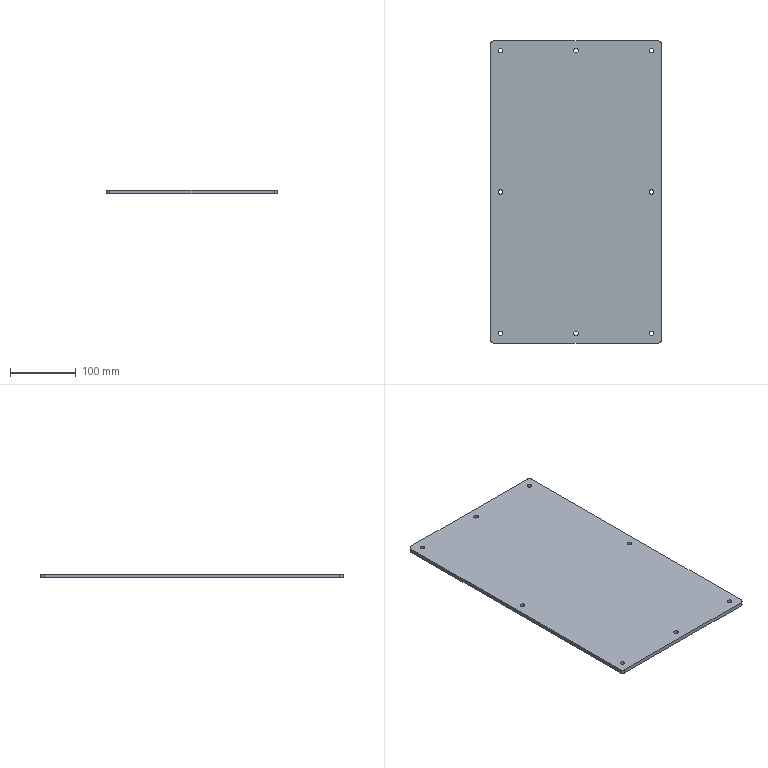Part | SolidWorks | features Extrusion 1, Fillet 1, ICE 1 | 1 solid | 26 faces | box 260 x 460 x 6 mm | volume 715624 mm3 | cylinder 20 | plane 6 | commonest cylinder face diameters 7 x16 10 x4
STEP:
#1=CARTESIAN_POINT('',(18.5,-230.,6.));
#2=VERTEX_POINT('',#1);
#3=CARTESIAN_POINT('',(11.5,-230.,6.));
#4=VERTEX_POINT('',#3);
#5=CARTESIAN_POINT('',(15.,-230.,6.));
#6=DIRECTION('',(0.,0.,-1.));
#7=DIRECTION('',(-1.,0.,0.));
#8=AXIS2_PLACEMENT_3D('',#5,#6,#7);
#9=CIRCLE('',#8,3.5);
#10=EDGE_CURVE('',#2,#4,#9,.T.);
#11=ORIENTED_EDGE('',*,*,#10,.F.);
#12=CARTESIAN_POINT('',(18.5,-230.,0.));
#13=VERTEX_POINT('',#12);
#14=CARTESIAN_POINT('',(18.5,-230.,6.));
#15=DIRECTION('',(0.,0.,-1.));
#16=VECTOR('',#15,1000.);
#17=LINE('',#14,#16);
#18=EDGE_CURVE('',#2,#13,#17,.T.);
#19=ORIENTED_EDGE('',*,*,#18,.T.);
#20=CARTESIAN_POINT('',(11.5,-230.,0.));
#21=VERTEX_POINT('',#20);
#22=CARTESIAN_POINT('',(15.,-230.,0.));
#23=DIRECTION('',(0.,0.,-1.));
#24=DIRECTION('',(-1.,0.,0.));
#25=AXIS2_PLACEMENT_3D('',#22,#23,#24);
#26=CIRCLE('',#25,3.5);
#27=EDGE_CURVE('',#13,#21,#26,.T.);
#28=ORIENTED_EDGE('',*,*,#27,.T.);
#29=CARTESIAN_POINT('',(11.5,-230.,6.));
#30=DIRECTION('',(0.,0.,-1.));
#31=VECTOR('',#30,1000.);
#32=LINE('',#29,#31);
#33=EDGE_CURVE('',#4,#21,#32,.T.);
#34=ORIENTED_EDGE('',*,*,#33,.F.);
#35=EDGE_LOOP('',(#11,#19,#28,#34));
#36=FACE_OUTER_BOUND('',#35,.T.);
#37=CARTESIAN_POINT('',(15.,-230.,6.));
#38=DIRECTION('',(0.,0.,-1.));
#39=DIRECTION('',(-1.,0.,0.));
#40=AXIS2_PLACEMENT_3D('',#37,#38,#39);
#41=CYLINDRICAL_SURFACE('',#40,3.5);
#42=ADVANCED_FACE('',(#36),#41,.F.);
#43=CARTESIAN_POINT('',(133.5,-15.,6.));
#44=VERTEX_POINT('',#43);
#45=CARTESIAN_POINT('',(126.5,-15.,6.));
#46=VERTEX_POINT('',#45);
#47=CARTESIAN_POINT('',(130.,-15.,6.));
#48=DIRECTION('',(0.,0.,-1.));
#49=DIRECTION('',(-1.,0.,0.));
#50=AXIS2_PLACEMENT_3D('',#47,#48,#49);
#51=CIRCLE('',#50,3.5);
#52=EDGE_CURVE('',#44,#46,#51,.T.);
#53=ORIENTED_EDGE('',*,*,#52,.F.);
#54=CARTESIAN_POINT('',(133.5,-15.,0.));
#55=VERTEX_POINT('',#54);
#56=CARTESIAN_POINT('',(133.5,-15.,6.));
#57=DIRECTION('',(0.,0.,-1.));
#58=VECTOR('',#57,1000.);
#59=LINE('',#56,#58);
#60=EDGE_CURVE('',#44,#55,#59,.T.);
#61=ORIENTED_EDGE('',*,*,#60,.T.);
#62=CARTESIAN_POINT('',(126.5,-15.,0.));
#63=VERTEX_POINT('',#62);
#64=CARTESIAN_POINT('',(130.,-15.,0.));
#65=DIRECTION('',(0.,0.,-1.));
#66=DIRECTION('',(-1.,0.,0.));
#67=AXIS2_PLACEMENT_3D('',#64,#65,#66);
#68=CIRCLE('',#67,3.5);
#69=EDGE_CURVE('',#55,#63,#68,.T.);
#70=ORIENTED_EDGE('',*,*,#69,.T.);
#71=CARTESIAN_POINT('',(126.5,-15.,6.));
#72=DIRECTION('',(0.,0.,-1.));
#73=VECTOR('',#72,1000.);
#74=LINE('',#71,#73);
#75=EDGE_CURVE('',#46,#63,#74,.T.);
#76=ORIENTED_EDGE('',*,*,#75,.F.);
#77=EDGE_LOOP('',(#53,#61,#70,#76));
#78=FACE_OUTER_BOUND('',#77,.T.);
#79=CARTESIAN_POINT('',(130.,-15.,6.));
#80=DIRECTION('',(0.,0.,-1.));
#81=DIRECTION('',(-1.,0.,0.));
#82=AXIS2_PLACEMENT_3D('',#79,#80,#81);
#83=CYLINDRICAL_SURFACE('',#82,3.5);
#84=ADVANCED_FACE('',(#78),#83,.F.);
#85=CARTESIAN_POINT('',(248.5,-230.,6.));
#86=VERTEX_POINT('',#85);
#87=CARTESIAN_POINT('',(241.5,-230.,6.));
#88=VERTEX_POINT('',#87);
#89=CARTESIAN_POINT('',(245.,-230.,6.));
#90=DIRECTION('',(0.,0.,-1.));
#91=DIRECTION('',(-1.,0.,0.));
#92=AXIS2_PLACEMENT_3D('',#89,#90,#91);
#93=CIRCLE('',#92,3.5);
#94=EDGE_CURVE('',#86,#88,#93,.T.);
#95=ORIENTED_EDGE('',*,*,#94,.F.);
#96=CARTESIAN_POINT('',(248.5,-230.,0.));
#97=VERTEX_POINT('',#96);
#98=CARTESIAN_POINT('',(248.5,-230.,6.));
#99=DIRECTION('',(0.,0.,-1.));
#100=VECTOR('',#99,1000.);
#101=LINE('',#98,#100);
#102=EDGE_CURVE('',#86,#97,#101,.T.);
#103=ORIENTED_EDGE('',*,*,#102,.T.);
#104=CARTESIAN_POINT('',(241.5,-230.,0.));
#105=VERTEX_POINT('',#104);
#106=CARTESIAN_POINT('',(245.,-230.,0.));
#107=DIRECTION('',(0.,0.,-1.));
#108=DIRECTION('',(-1.,0.,0.));
#109=AXIS2_PLACEMENT_3D('',#106,#107,#108);
#110=CIRCLE('',#109,3.5);
#111=EDGE_CURVE('',#97,#105,#110,.T.);
#112=ORIENTED_EDGE('',*,*,#111,.T.);
#113=CARTESIAN_POINT('',(241.5,-230.,6.));
#114=DIRECTION('',(0.,0.,-1.));
#115=VECTOR('',#114,1000.);
#116=LINE('',#113,#115);
#117=EDGE_CURVE('',#88,#105,#116,.T.);
#118=ORIENTED_EDGE('',*,*,#117,.F.);
#119=EDGE_LOOP('',(#95,#103,#112,#118));
#120=FACE_OUTER_BOUND('',#119,.T.);
#121=CARTESIAN_POINT('',(245.,-230.,6.));
#122=DIRECTION('',(0.,0.,-1.));
#123=DIRECTION('',(-1.,0.,0.));
#124=AXIS2_PLACEMENT_3D('',#121,#122,#123);
#125=CYLINDRICAL_SURFACE('',#124,3.5);
#126=ADVANCED_FACE('',(#120),#125,.F.);
#127=CARTESIAN_POINT('',(133.5,-445.,6.));
#128=VERTEX_POINT('',#127);
#129=CARTESIAN_POINT('',(126.5,-445.,6.));
#130=VERTEX_POINT('',#129);
#131=CARTESIAN_POINT('',(130.,-445.,6.));
#132=DIRECTION('',(0.,0.,-1.));
#133=DIRECTION('',(-1.,0.,0.));
#134=AXIS2_PLACEMENT_3D('',#131,#132,#133);
#135=CIRCLE('',#134,3.5);
#136=EDGE_CURVE('',#128,#130,#135,.T.);
#137=ORIENTED_EDGE('',*,*,#136,.F.);
#138=CARTESIAN_POINT('',(133.5,-445.,0.));
#139=VERTEX_POINT('',#138);
#140=CARTESIAN_POINT('',(133.5,-445.,6.));
#141=DIRECTION('',(0.,0.,-1.));
#142=VECTOR('',#141,1000.);
#143=LINE('',#140,#142);
#144=EDGE_CURVE('',#128,#139,#143,.T.);
#145=ORIENTED_EDGE('',*,*,#144,.T.);
#146=CARTESIAN_POINT('',(126.5,-445.,0.));
#147=VERTEX_POINT('',#146);
#148=CARTESIAN_POINT('',(130.,-445.,0.));
#149=DIRECTION('',(0.,0.,-1.));
#150=DIRECTION('',(-1.,0.,0.));
#151=AXIS2_PLACEMENT_3D('',#148,#149,#150);
#152=CIRCLE('',#151,3.5);
#153=EDGE_CURVE('',#139,#147,#152,.T.);
#154=ORIENTED_EDGE('',*,*,#153,.T.);
#155=CARTESIAN_POINT('',(126.5,-445.,6.));
#156=DIRECTION('',(0.,0.,-1.));
#157=VECTOR('',#156,1000.);
#158=LINE('',#155,#157);
#159=EDGE_CURVE('',#130,#147,#158,.T.);
#160=ORIENTED_EDGE('',*,*,#159,.F.);
#161=EDGE_LOOP('',(#137,#145,#154,#160));
#162=FACE_OUTER_BOUND('',#161,.T.);
#163=CARTESIAN_POINT('',(130.,-445.,6.));
#164=DIRECTION('',(0.,0.,-1.));
#165=DIRECTION('',(-1.,0.,0.));
#166=AXIS2_PLACEMENT_3D('',#163,#164,#165);
#167=CYLINDRICAL_SURFACE('',#166,3.5);
#168=ADVANCED_FACE('',(#162),#167,.F.);
#169=CARTESIAN_POINT('',(18.5,-15.,6.));
#170=VERTEX_POINT('',#169);
#171=CARTESIAN_POINT('',(11.5,-15.,6.));
#172=VERTEX_POINT('',#171);
#173=CARTESIAN_POINT('',(15.,-15.,6.));
#174=DIRECTION('',(0.,0.,-1.));
#175=DIRECTION('',(-1.,0.,0.));
#176=AXIS2_PLACEMENT_3D('',#173,#174,#175);
#177=CIRCLE('',#176,3.5);
#178=EDGE_CURVE('',#170,#172,#177,.T.);
#179=ORIENTED_EDGE('',*,*,#178,.F.);
#180=CARTESIAN_POINT('',(18.5,-15.,0.));
#181=VERTEX_POINT('',#180);
#182=CARTESIAN_POINT('',(18.5,-15.,6.));
#183=DIRECTION('',(0.,0.,-1.));
#184=VECTOR('',#183,1000.);
#185=LINE('',#182,#184);
#186=EDGE_CURVE('',#170,#181,#185,.T.);
#187=ORIENTED_EDGE('',*,*,#186,.T.);
#188=CARTESIAN_POINT('',(11.5,-15.,0.));
#189=VERTEX_POINT('',#188);
#190=CARTESIAN_POINT('',(15.,-15.,0.));
#191=DIRECTION('',(0.,0.,-1.));
#192=DIRECTION('',(-1.,0.,0.));
#193=AXIS2_PLACEMENT_3D('',#190,#191,#192);
#194=CIRCLE('',#193,3.5);
#195=EDGE_CURVE('',#181,#189,#194,.T.);
#196=ORIENTED_EDGE('',*,*,#195,.T.);
#197=CARTESIAN_POINT('',(11.5,-15.,6.));
#198=DIRECTION('',(0.,0.,-1.));
#199=VECTOR('',#198,1000.);
#200=LINE('',#197,#199);
#201=EDGE_CURVE('',#172,#189,#200,.T.);
#202=ORIENTED_EDGE('',*,*,#201,.F.);
#203=EDGE_LOOP('',(#179,#187,#196,#202));
#204=FACE_OUTER_BOUND('',#203,.T.);
#205=CARTESIAN_POINT('',(15.,-15.,6.));
#206=DIRECTION('',(0.,0.,-1.));
#207=DIRECTION('',(-1.,0.,0.));
#208=AXIS2_PLACEMENT_3D('',#205,#206,#207);
#209=CYLINDRICAL_SURFACE('',#208,3.5);
#210=ADVANCED_FACE('',(#204),#209,.F.);
#211=CARTESIAN_POINT('',(248.5,-15.,6.));
#212=VERTEX_POINT('',#211);
#213=CARTESIAN_POINT('',(241.5,-15.,6.));
#214=VERTEX_POINT('',#213);
#215=CARTESIAN_POINT('',(245.,-15.,6.));
#216=DIRECTION('',(0.,0.,-1.));
#217=DIRECTION('',(-1.,0.,0.));
#218=AXIS2_PLACEMENT_3D('',#215,#216,#217);
#219=CIRCLE('',#218,3.5);
#220=EDGE_CURVE('',#212,#214,#219,.T.);
#221=ORIENTED_EDGE('',*,*,#220,.F.);
#222=CARTESIAN_POINT('',(248.5,-15.,0.));
#223=VERTEX_POINT('',#222);
#224=CARTESIAN_POINT('',(248.5,-15.,6.));
#225=DIRECTION('',(0.,0.,-1.));
#226=VECTOR('',#225,1000.);
#227=LINE('',#224,#226);
#228=EDGE_CURVE('',#212,#223,#227,.T.);
#229=ORIENTED_EDGE('',*,*,#228,.T.);
#230=CARTESIAN_POINT('',(241.5,-15.,0.));
#231=VERTEX_POINT('',#230);
#232=CARTESIAN_POINT('',(245.,-15.,0.));
#233=DIRECTION('',(0.,0.,-1.));
#234=DIRECTION('',(-1.,0.,0.));
#235=AXIS2_PLACEMENT_3D('',#232,#233,#234);
#236=CIRCLE('',#235,3.5);
#237=EDGE_CURVE('',#223,#231,#236,.T.);
#238=ORIENTED_EDGE('',*,*,#237,.T.);
#239=CARTESIAN_POINT('',(241.5,-15.,6.));
#240=DIRECTION('',(0.,0.,-1.));
#241=VECTOR('',#240,1000.);
#242=LINE('',#239,#241);
#243=EDGE_CURVE('',#214,#231,#242,.T.);
#244=ORIENTED_EDGE('',*,*,#243,.F.);
#245=EDGE_LOOP('',(#221,#229,#238,#244));
#246=FACE_OUTER_BOUND('',#245,.T.);
#247=CARTESIAN_POINT('',(245.,-15.,6.));
#248=DIRECTION('',(0.,0.,-1.));
#249=DIRECTION('',(-1.,0.,0.));
#250=AXIS2_PLACEMENT_3D('',#247,#248,#249);
#251=CYLINDRICAL_SURFACE('',#250,3.5);
#252=ADVANCED_FACE('',(#246),#251,.F.);
#253=CARTESIAN_POINT('',(18.5,-445.,6.));
#254=VERTEX_POINT('',#253);
#255=CARTESIAN_POINT('',(11.5,-445.,6.));
#256=VERTEX_POINT('',#255);
#257=CARTESIAN_POINT('',(15.,-445.,6.));
#258=DIRECTION('',(0.,0.,-1.));
#259=DIRECTION('',(-1.,0.,0.));
#260=AXIS2_PLACEMENT_3D('',#257,#258,#259);
#261=CIRCLE('',#260,3.5);
#262=EDGE_CURVE('',#254,#256,#261,.T.);
#263=ORIENTED_EDGE('',*,*,#262,.F.);
#264=CARTESIAN_POINT('',(18.5,-445.,0.));
#265=VERTEX_POINT('',#264);
#266=CARTESIAN_POINT('',(18.5,-445.,6.));
#267=DIRECTION('',(0.,0.,-1.));
#268=VECTOR('',#267,1000.);
#269=LINE('',#266,#268);
#270=EDGE_CURVE('',#254,#265,#269,.T.);
#271=ORIENTED_EDGE('',*,*,#270,.T.);
#272=CARTESIAN_POINT('',(11.5,-445.,0.));
#273=VERTEX_POINT('',#272);
#274=CARTESIAN_POINT('',(15.,-445.,0.));
#275=DIRECTION('',(0.,0.,-1.));
#276=DIRECTION('',(-1.,0.,0.));
#277=AXIS2_PLACEMENT_3D('',#274,#275,#276);
#278=CIRCLE('',#277,3.5);
#279=EDGE_CURVE('',#265,#273,#278,.T.);
#280=ORIENTED_EDGE('',*,*,#279,.T.);
#281=CARTESIAN_POINT('',(11.5,-445.,6.));
#282=DIRECTION('',(0.,0.,-1.));
#283=VECTOR('',#282,1000.);
#284=LINE('',#281,#283);
#285=EDGE_CURVE('',#256,#273,#284,.T.);
#286=ORIENTED_EDGE('',*,*,#285,.F.);
#287=EDGE_LOOP('',(#263,#271,#280,#286));
#288=FACE_OUTER_BOUND('',#287,.T.);
#289=CARTESIAN_POINT('',(15.,-445.,6.));
#290=DIRECTION('',(0.,0.,-1.));
#291=DIRECTION('',(-1.,0.,0.));
#292=AXIS2_PLACEMENT_3D('',#289,#290,#291);
#293=CYLINDRICAL_SURFACE('',#292,3.5);
#294=ADVANCED_FACE('',(#288),#293,.F.);
#295=CARTESIAN_POINT('',(248.5,-445.,6.));
#296=VERTEX_POINT('',#295);
#297=CARTESIAN_POINT('',(241.5,-445.,6.));
#298=VERTEX_POINT('',#297);
#299=CARTESIAN_POINT('',(245.,-445.,6.));
#300=DIRECTION('',(0.,0.,-1.));
#301=DIRECTION('',(-1.,0.,0.));
#302=AXIS2_PLACEMENT_3D('',#299,#300,#301);
#303=CIRCLE('',#302,3.5);
#304=EDGE_CURVE('',#296,#298,#303,.T.);
#305=ORIENTED_EDGE('',*,*,#304,.F.);
#306=CARTESIAN_POINT('',(248.5,-445.,0.));
#307=VERTEX_POINT('',#306);
#308=CARTESIAN_POINT('',(248.5,-445.,6.));
#309=DIRECTION('',(0.,0.,-1.));
#310=VECTOR('',#309,1000.);
#311=LINE('',#308,#310);
#312=EDGE_CURVE('',#296,#307,#311,.T.);
#313=ORIENTED_EDGE('',*,*,#312,.T.);
#314=CARTESIAN_POINT('',(241.5,-445.,0.));
#315=VERTEX_POINT('',#314);
#316=CARTESIAN_POINT('',(245.,-445.,0.));
#317=DIRECTION('',(0.,0.,-1.));
#318=DIRECTION('',(-1.,0.,0.));
#319=AXIS2_PLACEMENT_3D('',#316,#317,#318);
#320=CIRCLE('',#319,3.5);
#321=EDGE_CURVE('',#307,#315,#320,.T.);
#322=ORIENTED_EDGE('',*,*,#321,.T.);
#323=CARTESIAN_POINT('',(241.5,-445.,6.));
#324=DIRECTION('',(0.,0.,-1.));
#325=VECTOR('',#324,1000.);
#326=LINE('',#323,#325);
#327=EDGE_CURVE('',#298,#315,#326,.T.);
#328=ORIENTED_EDGE('',*,*,#327,.F.);
#329=EDGE_LOOP('',(#305,#313,#322,#328));
#330=FACE_OUTER_BOUND('',#329,.T.);
#331=CARTESIAN_POINT('',(245.,-445.,6.));
#332=DIRECTION('',(0.,0.,-1.));
#333=DIRECTION('',(-1.,0.,0.));
#334=AXIS2_PLACEMENT_3D('',#331,#332,#333);
#335=CYLINDRICAL_SURFACE('',#334,3.5);
#336=ADVANCED_FACE('',(#330),#335,.F.);
#337=CARTESIAN_POINT('',(0.,-5.,0.));
#338=VERTEX_POINT('',#337);
#339=CARTESIAN_POINT('',(0.,-455.,0.));
#340=VERTEX_POINT('',#339);
#341=CARTESIAN_POINT('',(0.,0.,0.));
#342=DIRECTION('',(0.,-1.,0.));
#343=VECTOR('',#342,1000.);
#344=LINE('',#341,#343);
#345=EDGE_CURVE('',#338,#340,#344,.T.);
#346=ORIENTED_EDGE('',*,*,#345,.T.);
#347=CARTESIAN_POINT('',(0.,-455.,6.));
#348=VERTEX_POINT('',#347);
#349=CARTESIAN_POINT('',(0.,-455.,6.));
#350=DIRECTION('',(0.,0.,1.));
#351=VECTOR('',#350,1000.);
#352=LINE('',#349,#351);
#353=EDGE_CURVE('',#340,#348,#352,.T.);
#354=ORIENTED_EDGE('',*,*,#353,.T.);
#355=CARTESIAN_POINT('',(0.,-5.,6.));
#356=VERTEX_POINT('',#355);
#357=CARTESIAN_POINT('',(0.,0.,6.));
#358=DIRECTION('',(0.,-1.,0.));
#359=VECTOR('',#358,1000.);
#360=LINE('',#357,#359);
#361=EDGE_CURVE('',#356,#348,#360,.T.);
#362=ORIENTED_EDGE('',*,*,#361,.F.);
#363=CARTESIAN_POINT('',(0.,-5.,6.));
#364=DIRECTION('',(0.,0.,-1.));
#365=VECTOR('',#364,1000.);
#366=LINE('',#363,#365);
#367=EDGE_CURVE('',#356,#338,#366,.T.);
#368=ORIENTED_EDGE('',*,*,#367,.T.);
#369=EDGE_LOOP('',(#346,#354,#362,#368));
#370=FACE_OUTER_BOUND('',#369,.T.);
#371=CARTESIAN_POINT('',(0.,0.,6.));
#372=DIRECTION('',(1.,0.,0.));
#373=DIRECTION('',(0.,1.,0.));
#374=AXIS2_PLACEMENT_3D('',#371,#372,#373);
#375=PLANE('',#374);
#376=ADVANCED_FACE('',(#370),#375,.F.);
#377=CARTESIAN_POINT('',(5.,-460.,6.));
#378=VERTEX_POINT('',#377);
#379=CARTESIAN_POINT('',(255.,-460.,6.));
#380=VERTEX_POINT('',#379);
#381=CARTESIAN_POINT('',(0.,-460.,6.));
#382=DIRECTION('',(1.,0.,0.));
#383=VECTOR('',#382,1000.);
#384=LINE('',#381,#383);
#385=EDGE_CURVE('',#378,#380,#384,.T.);
#386=ORIENTED_EDGE('',*,*,#385,.F.);
#387=CARTESIAN_POINT('',(5.,-460.,0.));
#388=VERTEX_POINT('',#387);
#389=CARTESIAN_POINT('',(5.,-460.,6.));
#390=DIRECTION('',(0.,0.,-1.));
#391=VECTOR('',#390,1000.);
#392=LINE('',#389,#391);
#393=EDGE_CURVE('',#378,#388,#392,.T.);
#394=ORIENTED_EDGE('',*,*,#393,.T.);
#395=CARTESIAN_POINT('',(255.,-460.,0.));
#396=VERTEX_POINT('',#395);
#397=CARTESIAN_POINT('',(0.,-460.,0.));
#398=DIRECTION('',(1.,0.,0.));
#399=VECTOR('',#398,1000.);
#400=LINE('',#397,#399);
#401=EDGE_CURVE('',#388,#396,#400,.T.);
#402=ORIENTED_EDGE('',*,*,#401,.T.);
#403=CARTESIAN_POINT('',(255.,-460.,6.));
#404=DIRECTION('',(0.,0.,1.));
#405=VECTOR('',#404,1000.);
#406=LINE('',#403,#405);
#407=EDGE_CURVE('',#396,#380,#406,.T.);
#408=ORIENTED_EDGE('',*,*,#407,.T.);
#409=EDGE_LOOP('',(#386,#394,#402,#408));
#410=FACE_OUTER_BOUND('',#409,.T.);
#411=CARTESIAN_POINT('',(0.,-460.,6.));
#412=DIRECTION('',(0.,1.,0.));
#413=DIRECTION('',(0.,0.,1.));
#414=AXIS2_PLACEMENT_3D('',#411,#412,#413);
#415=PLANE('',#414);
#416=ADVANCED_FACE('',(#410),#415,.F.);
#417=CARTESIAN_POINT('',(260.,-455.,6.));
#418=VERTEX_POINT('',#417);
#419=CARTESIAN_POINT('',(260.,-5.,6.));
#420=VERTEX_POINT('',#419);
#421=CARTESIAN_POINT('',(260.,0.,6.));
#422=DIRECTION('',(0.,1.,0.));
#423=VECTOR('',#422,1000.);
#424=LINE('',#421,#423);
#425=EDGE_CURVE('',#418,#420,#424,.T.);
#426=ORIENTED_EDGE('',*,*,#425,.F.);
#427=CARTESIAN_POINT('',(260.,-455.,0.));
#428=VERTEX_POINT('',#427);
#429=CARTESIAN_POINT('',(260.,-455.,6.));
#430=DIRECTION('',(0.,0.,-1.));
#431=VECTOR('',#430,1000.);
#432=LINE('',#429,#431);
#433=EDGE_CURVE('',#418,#428,#432,.T.);
#434=ORIENTED_EDGE('',*,*,#433,.T.);
#435=CARTESIAN_POINT('',(260.,-5.,0.));
#436=VERTEX_POINT('',#435);
#437=CARTESIAN_POINT('',(260.,0.,0.));
#438=DIRECTION('',(0.,1.,0.));
#439=VECTOR('',#438,1000.);
#440=LINE('',#437,#439);
#441=EDGE_CURVE('',#428,#436,#440,.T.);
#442=ORIENTED_EDGE('',*,*,#441,.T.);
#443=CARTESIAN_POINT('',(260.,-5.,6.));
#444=DIRECTION('',(0.,0.,1.));
#445=VECTOR('',#444,1000.);
#446=LINE('',#443,#445);
#447=EDGE_CURVE('',#436,#420,#446,.T.);
#448=ORIENTED_EDGE('',*,*,#447,.T.);
#449=EDGE_LOOP('',(#426,#434,#442,#448));
#450=FACE_OUTER_BOUND('',#449,.T.);
#451=CARTESIAN_POINT('',(260.,0.,6.));
#452=DIRECTION('',(-1.,0.,0.));
#453=DIRECTION('',(0.,0.,1.));
#454=AXIS2_PLACEMENT_3D('',#451,#452,#453);
#455=PLANE('',#454);
#456=ADVANCED_FACE('',(#450),#455,.F.);
#457=CARTESIAN_POINT('',(255.,0.,6.));
#458=VERTEX_POINT('',#457);
#459=CARTESIAN_POINT('',(5.,0.,6.));
#460=VERTEX_POINT('',#459);
#461=CARTESIAN_POINT('',(0.,0.,6.));
#462=DIRECTION('',(-1.,0.,0.));
#463=VECTOR('',#462,1000.);
#464=LINE('',#461,#463);
#465=EDGE_CURVE('',#458,#460,#464,.T.);
#466=ORIENTED_EDGE('',*,*,#465,.F.);
#467=CARTESIAN_POINT('',(255.,0.,0.));
#468=VERTEX_POINT('',#467);
#469=CARTESIAN_POINT('',(255.,0.,6.));
#470=DIRECTION('',(0.,0.,-1.));
#471=VECTOR('',#470,1000.);
#472=LINE('',#469,#471);
#473=EDGE_CURVE('',#458,#468,#472,.T.);
#474=ORIENTED_EDGE('',*,*,#473,.T.);
#475=CARTESIAN_POINT('',(5.,0.,0.));
#476=VERTEX_POINT('',#475);
#477=CARTESIAN_POINT('',(0.,0.,0.));
#478=DIRECTION('',(-1.,0.,0.));
#479=VECTOR('',#478,1000.);
#480=LINE('',#477,#479);
#481=EDGE_CURVE('',#468,#476,#480,.T.);
#482=ORIENTED_EDGE('',*,*,#481,.T.);
#483=CARTESIAN_POINT('',(5.,0.,6.));
#484=DIRECTION('',(0.,0.,1.));
#485=VECTOR('',#484,1000.);
#486=LINE('',#483,#485);
#487=EDGE_CURVE('',#476,#460,#486,.T.);
#488=ORIENTED_EDGE('',*,*,#487,.T.);
#489=EDGE_LOOP('',(#466,#474,#482,#488));
#490=FACE_OUTER_BOUND('',#489,.T.);
#491=CARTESIAN_POINT('',(0.,0.,6.));
#492=DIRECTION('',(0.,-1.,0.));
#493=DIRECTION('',(0.,0.,-1.));
#494=AXIS2_PLACEMENT_3D('',#491,#492,#493);
#495=PLANE('',#494);
#496=ADVANCED_FACE('',(#490),#495,.F.);
#497=CARTESIAN_POINT('',(15.,-230.,6.));
#498=DIRECTION('',(0.,0.,-1.));
#499=DIRECTION('',(-1.,0.,0.));
#500=AXIS2_PLACEMENT_3D('',#497,#498,#499);
#501=CIRCLE('',#500,3.5);
#502=EDGE_CURVE('',#4,#2,#501,.T.);
#503=ORIENTED_EDGE('',*,*,#502,.T.);
#504=ORIENTED_EDGE('',*,*,#10,.T.);
#505=EDGE_LOOP('',(#503,#504));
#506=FACE_BOUND('',#505,.T.);
#507=CARTESIAN_POINT('',(130.,-15.,6.));
#508=DIRECTION('',(0.,0.,-1.));
#509=DIRECTION('',(-1.,0.,0.));
#510=AXIS2_PLACEMENT_3D('',#507,#508,#509);
#511=CIRCLE('',#510,3.5);
#512=EDGE_CURVE('',#46,#44,#511,.T.);
#513=ORIENTED_EDGE('',*,*,#512,.T.);
#514=ORIENTED_EDGE('',*,*,#52,.T.);
#515=EDGE_LOOP('',(#513,#514));
#516=FACE_BOUND('',#515,.T.);
#517=CARTESIAN_POINT('',(245.,-230.,6.));
#518=DIRECTION('',(0.,0.,-1.));
#519=DIRECTION('',(-1.,0.,0.));
#520=AXIS2_PLACEMENT_3D('',#517,#518,#519);
#521=CIRCLE('',#520,3.5);
#522=EDGE_CURVE('',#88,#86,#521,.T.);
#523=ORIENTED_EDGE('',*,*,#522,.T.);
#524=ORIENTED_EDGE('',*,*,#94,.T.);
#525=EDGE_LOOP('',(#523,#524));
#526=FACE_BOUND('',#525,.T.);
#527=CARTESIAN_POINT('',(130.,-445.,6.));
#528=DIRECTION('',(0.,0.,-1.));
#529=DIRECTION('',(-1.,0.,0.));
#530=AXIS2_PLACEMENT_3D('',#527,#528,#529);
#531=CIRCLE('',#530,3.5);
#532=EDGE_CURVE('',#130,#128,#531,.T.);
#533=ORIENTED_EDGE('',*,*,#532,.T.);
#534=ORIENTED_EDGE('',*,*,#136,.T.);
#535=EDGE_LOOP('',(#533,#534));
#536=FACE_BOUND('',#535,.T.);
#537=CARTESIAN_POINT('',(15.,-15.,6.));
#538=DIRECTION('',(0.,0.,-1.));
#539=DIRECTION('',(-1.,0.,0.));
#540=AXIS2_PLACEMENT_3D('',#537,#538,#539);
#541=CIRCLE('',#540,3.5);
#542=EDGE_CURVE('',#172,#170,#541,.T.);
#543=ORIENTED_EDGE('',*,*,#542,.T.);
#544=ORIENTED_EDGE('',*,*,#178,.T.);
#545=EDGE_LOOP('',(#543,#544));
#546=FACE_BOUND('',#545,.T.);
#547=CARTESIAN_POINT('',(245.,-15.,6.));
#548=DIRECTION('',(0.,0.,-1.));
#549=DIRECTION('',(-1.,0.,0.));
#550=AXIS2_PLACEMENT_3D('',#547,#548,#549);
#551=CIRCLE('',#550,3.5);
#552=EDGE_CURVE('',#214,#212,#551,.T.);
#553=ORIENTED_EDGE('',*,*,#552,.T.);
#554=ORIENTED_EDGE('',*,*,#220,.T.);
#555=EDGE_LOOP('',(#553,#554));
#556=FACE_BOUND('',#555,.T.);
#557=CARTESIAN_POINT('',(15.,-445.,6.));
#558=DIRECTION('',(0.,0.,-1.));
#559=DIRECTION('',(-1.,0.,0.));
#560=AXIS2_PLACEMENT_3D('',#557,#558,#559);
#561=CIRCLE('',#560,3.5);
#562=EDGE_CURVE('',#256,#254,#561,.T.);
#563=ORIENTED_EDGE('',*,*,#562,.T.);
#564=ORIENTED_EDGE('',*,*,#262,.T.);
#565=EDGE_LOOP('',(#563,#564));
#566=FACE_BOUND('',#565,.T.);
#567=CARTESIAN_POINT('',(245.,-445.,6.));
#568=DIRECTION('',(0.,0.,-1.));
#569=DIRECTION('',(-1.,0.,0.));
#570=AXIS2_PLACEMENT_3D('',#567,#568,#569);
#571=CIRCLE('',#570,3.5);
#572=EDGE_CURVE('',#298,#296,#571,.T.);
#573=ORIENTED_EDGE('',*,*,#572,.T.);
#574=ORIENTED_EDGE('',*,*,#304,.T.);
#575=EDGE_LOOP('',(#573,#574));
#576=FACE_BOUND('',#575,.T.);
#577=ORIENTED_EDGE('',*,*,#361,.T.);
#578=CARTESIAN_POINT('',(5.,-455.,6.));
#579=DIRECTION('',(0.,0.,1.));
#580=DIRECTION('',(1.,0.,0.));
#581=AXIS2_PLACEMENT_3D('',#578,#579,#580);
#582=CIRCLE('',#581,5.);
#583=EDGE_CURVE('',#348,#378,#582,.T.);
#584=ORIENTED_EDGE('',*,*,#583,.T.);
#585=ORIENTED_EDGE('',*,*,#385,.T.);
#586=CARTESIAN_POINT('',(255.,-455.,6.));
#587=DIRECTION('',(0.,0.,1.));
#588=DIRECTION('',(1.,0.,0.));
#589=AXIS2_PLACEMENT_3D('',#586,#587,#588);
#590=CIRCLE('',#589,5.);
#591=EDGE_CURVE('',#380,#418,#590,.T.);
#592=ORIENTED_EDGE('',*,*,#591,.T.);
#593=ORIENTED_EDGE('',*,*,#425,.T.);
#594=CARTESIAN_POINT('',(255.,-5.,6.));
#595=DIRECTION('',(0.,0.,1.));
#596=DIRECTION('',(1.,0.,0.));
#597=AXIS2_PLACEMENT_3D('',#594,#595,#596);
#598=CIRCLE('',#597,5.);
#599=EDGE_CURVE('',#420,#458,#598,.T.);
#600=ORIENTED_EDGE('',*,*,#599,.T.);
#601=ORIENTED_EDGE('',*,*,#465,.T.);
#602=CARTESIAN_POINT('',(5.,-5.,6.));
#603=DIRECTION('',(0.,0.,1.));
#604=DIRECTION('',(1.,0.,0.));
#605=AXIS2_PLACEMENT_3D('',#602,#603,#604);
#606=CIRCLE('',#605,5.);
#607=EDGE_CURVE('',#460,#356,#606,.T.);
#608=ORIENTED_EDGE('',*,*,#607,.T.);
#609=EDGE_LOOP('',(#577,#584,#585,#592,#593,#600,#601,#608));
#610=FACE_OUTER_BOUND('',#609,.T.);
#611=CARTESIAN_POINT('',(0.,0.,6.));
#612=DIRECTION('',(0.,0.,1.));
#613=DIRECTION('',(1.,0.,0.));
#614=AXIS2_PLACEMENT_3D('',#611,#612,#613);
#615=PLANE('',#614);
#616=ADVANCED_FACE('',(#506,#516,#526,#536,#546,#556,#566,#576,#610),#615,.T.);
#617=CARTESIAN_POINT('',(15.,-230.,0.));
#618=DIRECTION('',(0.,0.,-1.));
#619=DIRECTION('',(-1.,0.,0.));
#620=AXIS2_PLACEMENT_3D('',#617,#618,#619);
#621=CIRCLE('',#620,3.5);
#622=EDGE_CURVE('',#21,#13,#621,.T.);
#623=ORIENTED_EDGE('',*,*,#622,.F.);
#624=ORIENTED_EDGE('',*,*,#27,.F.);
#625=EDGE_LOOP('',(#623,#624));
#626=FACE_BOUND('',#625,.T.);
#627=CARTESIAN_POINT('',(130.,-15.,0.));
#628=DIRECTION('',(0.,0.,-1.));
#629=DIRECTION('',(-1.,0.,0.));
#630=AXIS2_PLACEMENT_3D('',#627,#628,#629);
#631=CIRCLE('',#630,3.5);
#632=EDGE_CURVE('',#63,#55,#631,.T.);
#633=ORIENTED_EDGE('',*,*,#632,.F.);
#634=ORIENTED_EDGE('',*,*,#69,.F.);
#635=EDGE_LOOP('',(#633,#634));
#636=FACE_BOUND('',#635,.T.);
#637=CARTESIAN_POINT('',(245.,-230.,0.));
#638=DIRECTION('',(0.,0.,-1.));
#639=DIRECTION('',(-1.,0.,0.));
#640=AXIS2_PLACEMENT_3D('',#637,#638,#639);
#641=CIRCLE('',#640,3.5);
#642=EDGE_CURVE('',#105,#97,#641,.T.);
#643=ORIENTED_EDGE('',*,*,#642,.F.);
#644=ORIENTED_EDGE('',*,*,#111,.F.);
#645=EDGE_LOOP('',(#643,#644));
#646=FACE_BOUND('',#645,.T.);
#647=CARTESIAN_POINT('',(130.,-445.,0.));
#648=DIRECTION('',(0.,0.,-1.));
#649=DIRECTION('',(-1.,0.,0.));
#650=AXIS2_PLACEMENT_3D('',#647,#648,#649);
#651=CIRCLE('',#650,3.5);
#652=EDGE_CURVE('',#147,#139,#651,.T.);
#653=ORIENTED_EDGE('',*,*,#652,.F.);
#654=ORIENTED_EDGE('',*,*,#153,.F.);
#655=EDGE_LOOP('',(#653,#654));
#656=FACE_BOUND('',#655,.T.);
#657=CARTESIAN_POINT('',(15.,-15.,0.));
#658=DIRECTION('',(0.,0.,-1.));
#659=DIRECTION('',(-1.,0.,0.));
#660=AXIS2_PLACEMENT_3D('',#657,#658,#659);
#661=CIRCLE('',#660,3.5);
#662=EDGE_CURVE('',#189,#181,#661,.T.);
#663=ORIENTED_EDGE('',*,*,#662,.F.);
#664=ORIENTED_EDGE('',*,*,#195,.F.);
#665=EDGE_LOOP('',(#663,#664));
#666=FACE_BOUND('',#665,.T.);
#667=CARTESIAN_POINT('',(245.,-15.,0.));
#668=DIRECTION('',(0.,0.,-1.));
#669=DIRECTION('',(-1.,0.,0.));
#670=AXIS2_PLACEMENT_3D('',#667,#668,#669);
#671=CIRCLE('',#670,3.5);
#672=EDGE_CURVE('',#231,#223,#671,.T.);
#673=ORIENTED_EDGE('',*,*,#672,.F.);
#674=ORIENTED_EDGE('',*,*,#237,.F.);
#675=EDGE_LOOP('',(#673,#674));
#676=FACE_BOUND('',#675,.T.);
#677=CARTESIAN_POINT('',(15.,-445.,0.));
#678=DIRECTION('',(0.,0.,-1.));
#679=DIRECTION('',(-1.,0.,0.));
#680=AXIS2_PLACEMENT_3D('',#677,#678,#679);
#681=CIRCLE('',#680,3.5);
#682=EDGE_CURVE('',#273,#265,#681,.T.);
#683=ORIENTED_EDGE('',*,*,#682,.F.);
#684=ORIENTED_EDGE('',*,*,#279,.F.);
#685=EDGE_LOOP('',(#683,#684));
#686=FACE_BOUND('',#685,.T.);
#687=CARTESIAN_POINT('',(245.,-445.,0.));
#688=DIRECTION('',(0.,0.,-1.));
#689=DIRECTION('',(-1.,0.,0.));
#690=AXIS2_PLACEMENT_3D('',#687,#688,#689);
#691=CIRCLE('',#690,3.5);
#692=EDGE_CURVE('',#315,#307,#691,.T.);
#693=ORIENTED_EDGE('',*,*,#692,.F.);
#694=ORIENTED_EDGE('',*,*,#321,.F.);
#695=EDGE_LOOP('',(#693,#694));
#696=FACE_BOUND('',#695,.T.);
#697=ORIENTED_EDGE('',*,*,#401,.F.);
#698=CARTESIAN_POINT('',(5.,-455.,0.));
#699=DIRECTION('',(0.,0.,-1.));
#700=DIRECTION('',(1.,0.,0.));
#701=AXIS2_PLACEMENT_3D('',#698,#699,#700);
#702=CIRCLE('',#701,5.);
#703=EDGE_CURVE('',#388,#340,#702,.T.);
#704=ORIENTED_EDGE('',*,*,#703,.T.);
#705=ORIENTED_EDGE('',*,*,#345,.F.);
#706=CARTESIAN_POINT('',(5.,-5.,0.));
#707=DIRECTION('',(0.,0.,-1.));
#708=DIRECTION('',(1.,0.,0.));
#709=AXIS2_PLACEMENT_3D('',#706,#707,#708);
#710=CIRCLE('',#709,5.);
#711=EDGE_CURVE('',#338,#476,#710,.T.);
#712=ORIENTED_EDGE('',*,*,#711,.T.);
#713=ORIENTED_EDGE('',*,*,#481,.F.);
#714=CARTESIAN_POINT('',(255.,-5.,0.));
#715=DIRECTION('',(0.,0.,-1.));
#716=DIRECTION('',(1.,0.,0.));
#717=AXIS2_PLACEMENT_3D('',#714,#715,#716);
#718=CIRCLE('',#717,5.);
#719=EDGE_CURVE('',#468,#436,#718,.T.);
#720=ORIENTED_EDGE('',*,*,#719,.T.);
#721=ORIENTED_EDGE('',*,*,#441,.F.);
#722=CARTESIAN_POINT('',(255.,-455.,0.));
#723=DIRECTION('',(0.,0.,-1.));
#724=DIRECTION('',(1.,0.,0.));
#725=AXIS2_PLACEMENT_3D('',#722,#723,#724);
#726=CIRCLE('',#725,5.);
#727=EDGE_CURVE('',#428,#396,#726,.T.);
#728=ORIENTED_EDGE('',*,*,#727,.T.);
#729=EDGE_LOOP('',(#697,#704,#705,#712,#713,#720,#721,#728));
#730=FACE_OUTER_BOUND('',#729,.T.);
#731=CARTESIAN_POINT('',(0.,0.,0.));
#732=DIRECTION('',(0.,0.,1.));
#733=DIRECTION('',(1.,0.,0.));
#734=AXIS2_PLACEMENT_3D('',#731,#732,#733);
#735=PLANE('',#734);
#736=ADVANCED_FACE('',(#626,#636,#646,#656,#666,#676,#686,#696,#730),#735,.F.);
#737=ORIENTED_EDGE('',*,*,#583,.F.);
#738=ORIENTED_EDGE('',*,*,#353,.F.);
#739=ORIENTED_EDGE('',*,*,#703,.F.);
#740=ORIENTED_EDGE('',*,*,#393,.F.);
#741=EDGE_LOOP('',(#737,#738,#739,#740));
#742=FACE_OUTER_BOUND('',#741,.T.);
#743=CARTESIAN_POINT('',(5.,-455.,6.));
#744=DIRECTION('',(0.,0.,-1.));
#745=DIRECTION('',(-1.,0.,0.));
#746=AXIS2_PLACEMENT_3D('',#743,#744,#745);
#747=CYLINDRICAL_SURFACE('',#746,5.);
#748=ADVANCED_FACE('',(#742),#747,.T.);
#749=ORIENTED_EDGE('',*,*,#591,.F.);
#750=ORIENTED_EDGE('',*,*,#407,.F.);
#751=ORIENTED_EDGE('',*,*,#727,.F.);
#752=ORIENTED_EDGE('',*,*,#433,.F.);
#753=EDGE_LOOP('',(#749,#750,#751,#752));
#754=FACE_OUTER_BOUND('',#753,.T.);
#755=CARTESIAN_POINT('',(255.,-455.,6.));
#756=DIRECTION('',(0.,0.,-1.));
#757=DIRECTION('',(-1.,0.,0.));
#758=AXIS2_PLACEMENT_3D('',#755,#756,#757);
#759=CYLINDRICAL_SURFACE('',#758,5.);
#760=ADVANCED_FACE('',(#754),#759,.T.);
#761=ORIENTED_EDGE('',*,*,#599,.F.);
#762=ORIENTED_EDGE('',*,*,#447,.F.);
#763=ORIENTED_EDGE('',*,*,#719,.F.);
#764=ORIENTED_EDGE('',*,*,#473,.F.);
#765=EDGE_LOOP('',(#761,#762,#763,#764));
#766=FACE_OUTER_BOUND('',#765,.T.);
#767=CARTESIAN_POINT('',(255.,-5.,6.));
#768=DIRECTION('',(0.,0.,-1.));
#769=DIRECTION('',(-1.,0.,0.));
#770=AXIS2_PLACEMENT_3D('',#767,#768,#769);
#771=CYLINDRICAL_SURFACE('',#770,5.);
#772=ADVANCED_FACE('',(#766),#771,.T.);
#773=ORIENTED_EDGE('',*,*,#607,.F.);
#774=ORIENTED_EDGE('',*,*,#487,.F.);
#775=ORIENTED_EDGE('',*,*,#711,.F.);
#776=ORIENTED_EDGE('',*,*,#367,.F.);
#777=EDGE_LOOP('',(#773,#774,#775,#776));
#778=FACE_OUTER_BOUND('',#777,.T.);
#779=CARTESIAN_POINT('',(5.,-5.,6.));
#780=DIRECTION('',(0.,0.,-1.));
#781=DIRECTION('',(-1.,0.,0.));
#782=AXIS2_PLACEMENT_3D('',#779,#780,#781);
#783=CYLINDRICAL_SURFACE('',#782,5.);
#784=ADVANCED_FACE('',(#778),#783,.T.);
#785=ORIENTED_EDGE('',*,*,#312,.F.);
#786=ORIENTED_EDGE('',*,*,#572,.F.);
#787=ORIENTED_EDGE('',*,*,#327,.T.);
#788=ORIENTED_EDGE('',*,*,#692,.T.);
#789=EDGE_LOOP('',(#785,#786,#787,#788));
#790=FACE_OUTER_BOUND('',#789,.T.);
#791=CARTESIAN_POINT('',(245.,-445.,6.));
#792=DIRECTION('',(0.,0.,-1.));
#793=DIRECTION('',(-1.,0.,0.));
#794=AXIS2_PLACEMENT_3D('',#791,#792,#793);
#795=CYLINDRICAL_SURFACE('',#794,3.5);
#796=ADVANCED_FACE('',(#790),#795,.F.);
#797=ORIENTED_EDGE('',*,*,#270,.F.);
#798=ORIENTED_EDGE('',*,*,#562,.F.);
#799=ORIENTED_EDGE('',*,*,#285,.T.);
#800=ORIENTED_EDGE('',*,*,#682,.T.);
#801=EDGE_LOOP('',(#797,#798,#799,#800));
#802=FACE_OUTER_BOUND('',#801,.T.);
#803=CARTESIAN_POINT('',(15.,-445.,6.));
#804=DIRECTION('',(0.,0.,-1.));
#805=DIRECTION('',(-1.,0.,0.));
#806=AXIS2_PLACEMENT_3D('',#803,#804,#805);
#807=CYLINDRICAL_SURFACE('',#806,3.5);
#808=ADVANCED_FACE('',(#802),#807,.F.);
#809=ORIENTED_EDGE('',*,*,#228,.F.);
#810=ORIENTED_EDGE('',*,*,#552,.F.);
#811=ORIENTED_EDGE('',*,*,#243,.T.);
#812=ORIENTED_EDGE('',*,*,#672,.T.);
#813=EDGE_LOOP('',(#809,#810,#811,#812));
#814=FACE_OUTER_BOUND('',#813,.T.);
#815=CARTESIAN_POINT('',(245.,-15.,6.));
#816=DIRECTION('',(0.,0.,-1.));
#817=DIRECTION('',(-1.,0.,0.));
#818=AXIS2_PLACEMENT_3D('',#815,#816,#817);
#819=CYLINDRICAL_SURFACE('',#818,3.5);
#820=ADVANCED_FACE('',(#814),#819,.F.);
#821=ORIENTED_EDGE('',*,*,#186,.F.);
#822=ORIENTED_EDGE('',*,*,#542,.F.);
#823=ORIENTED_EDGE('',*,*,#201,.T.);
#824=ORIENTED_EDGE('',*,*,#662,.T.);
#825=EDGE_LOOP('',(#821,#822,#823,#824));
#826=FACE_OUTER_BOUND('',#825,.T.);
#827=CARTESIAN_POINT('',(15.,-15.,6.));
#828=DIRECTION('',(0.,0.,-1.));
#829=DIRECTION('',(-1.,0.,0.));
#830=AXIS2_PLACEMENT_3D('',#827,#828,#829);
#831=CYLINDRICAL_SURFACE('',#830,3.5);
#832=ADVANCED_FACE('',(#826),#831,.F.);
#833=ORIENTED_EDGE('',*,*,#144,.F.);
#834=ORIENTED_EDGE('',*,*,#532,.F.);
#835=ORIENTED_EDGE('',*,*,#159,.T.);
#836=ORIENTED_EDGE('',*,*,#652,.T.);
#837=EDGE_LOOP('',(#833,#834,#835,#836));
#838=FACE_OUTER_BOUND('',#837,.T.);
#839=CARTESIAN_POINT('',(130.,-445.,6.));
#840=DIRECTION('',(0.,0.,-1.));
#841=DIRECTION('',(-1.,0.,0.));
#842=AXIS2_PLACEMENT_3D('',#839,#840,#841);
#843=CYLINDRICAL_SURFACE('',#842,3.5);
#844=ADVANCED_FACE('',(#838),#843,.F.);
#845=ORIENTED_EDGE('',*,*,#102,.F.);
#846=ORIENTED_EDGE('',*,*,#522,.F.);
#847=ORIENTED_EDGE('',*,*,#117,.T.);
#848=ORIENTED_EDGE('',*,*,#642,.T.);
#849=EDGE_LOOP('',(#845,#846,#847,#848));
#850=FACE_OUTER_BOUND('',#849,.T.);
#851=CARTESIAN_POINT('',(245.,-230.,6.));
#852=DIRECTION('',(0.,0.,-1.));
#853=DIRECTION('',(-1.,0.,0.));
#854=AXIS2_PLACEMENT_3D('',#851,#852,#853);
#855=CYLINDRICAL_SURFACE('',#854,3.5);
#856=ADVANCED_FACE('',(#850),#855,.F.);
#857=ORIENTED_EDGE('',*,*,#60,.F.);
#858=ORIENTED_EDGE('',*,*,#512,.F.);
#859=ORIENTED_EDGE('',*,*,#75,.T.);
#860=ORIENTED_EDGE('',*,*,#632,.T.);
#861=EDGE_LOOP('',(#857,#858,#859,#860));
#862=FACE_OUTER_BOUND('',#861,.T.);
#863=CARTESIAN_POINT('',(130.,-15.,6.));
#864=DIRECTION('',(0.,0.,-1.));
#865=DIRECTION('',(-1.,0.,0.));
#866=AXIS2_PLACEMENT_3D('',#863,#864,#865);
#867=CYLINDRICAL_SURFACE('',#866,3.5);
#868=ADVANCED_FACE('',(#862),#867,.F.);
#869=ORIENTED_EDGE('',*,*,#18,.F.);
#870=ORIENTED_EDGE('',*,*,#502,.F.);
#871=ORIENTED_EDGE('',*,*,#33,.T.);
#872=ORIENTED_EDGE('',*,*,#622,.T.);
#873=EDGE_LOOP('',(#869,#870,#871,#872));
#874=FACE_OUTER_BOUND('',#873,.T.);
#875=CARTESIAN_POINT('',(15.,-230.,6.));
#876=DIRECTION('',(0.,0.,-1.));
#877=DIRECTION('',(-1.,0.,0.));
#878=AXIS2_PLACEMENT_3D('',#875,#876,#877);
#879=CYLINDRICAL_SURFACE('',#878,3.5);
#880=ADVANCED_FACE('',(#874),#879,.F.);
#881=CLOSED_SHELL('',(#42,#84,#126,#168,#210,#252,#294,#336,#376,#416,#456,#496,#616,#736,#748,#760,#772,#784,#796,#808,#820,#832,#844,#856,#868,#880));
#882=MANIFOLD_SOLID_BREP('',#881);
#883=CARTESIAN_POINT('',(0.,0.,0.));
#884=DIRECTION('',(0.,0.,1.));
#885=DIRECTION('',(1.,0.,0.));
#886=AXIS2_PLACEMENT_3D('',#883,#884,#885);
#887=(LENGTH_UNIT()NAMED_UNIT(*)SI_UNIT(.MILLI.,.METRE.));
#888=UNCERTAINTY_MEASURE_WITH_UNIT(LENGTH_MEASURE(0.00001),#887,'','');
#889=(NAMED_UNIT(*)PLANE_ANGLE_UNIT()SI_UNIT($,.RADIAN.));
#890=(NAMED_UNIT(*)SI_UNIT($,.STERADIAN.)SOLID_ANGLE_UNIT());
#891=(GEOMETRIC_REPRESENTATION_CONTEXT(3)GLOBAL_UNCERTAINTY_ASSIGNED_CONTEXT((#888))GLOBAL_UNIT_ASSIGNED_CONTEXT((#887,#889,#890))REPRESENTATION_CONTEXT('',''));
#892=ADVANCED_BREP_SHAPE_REPRESENTATION('',(#882,#886),#891);